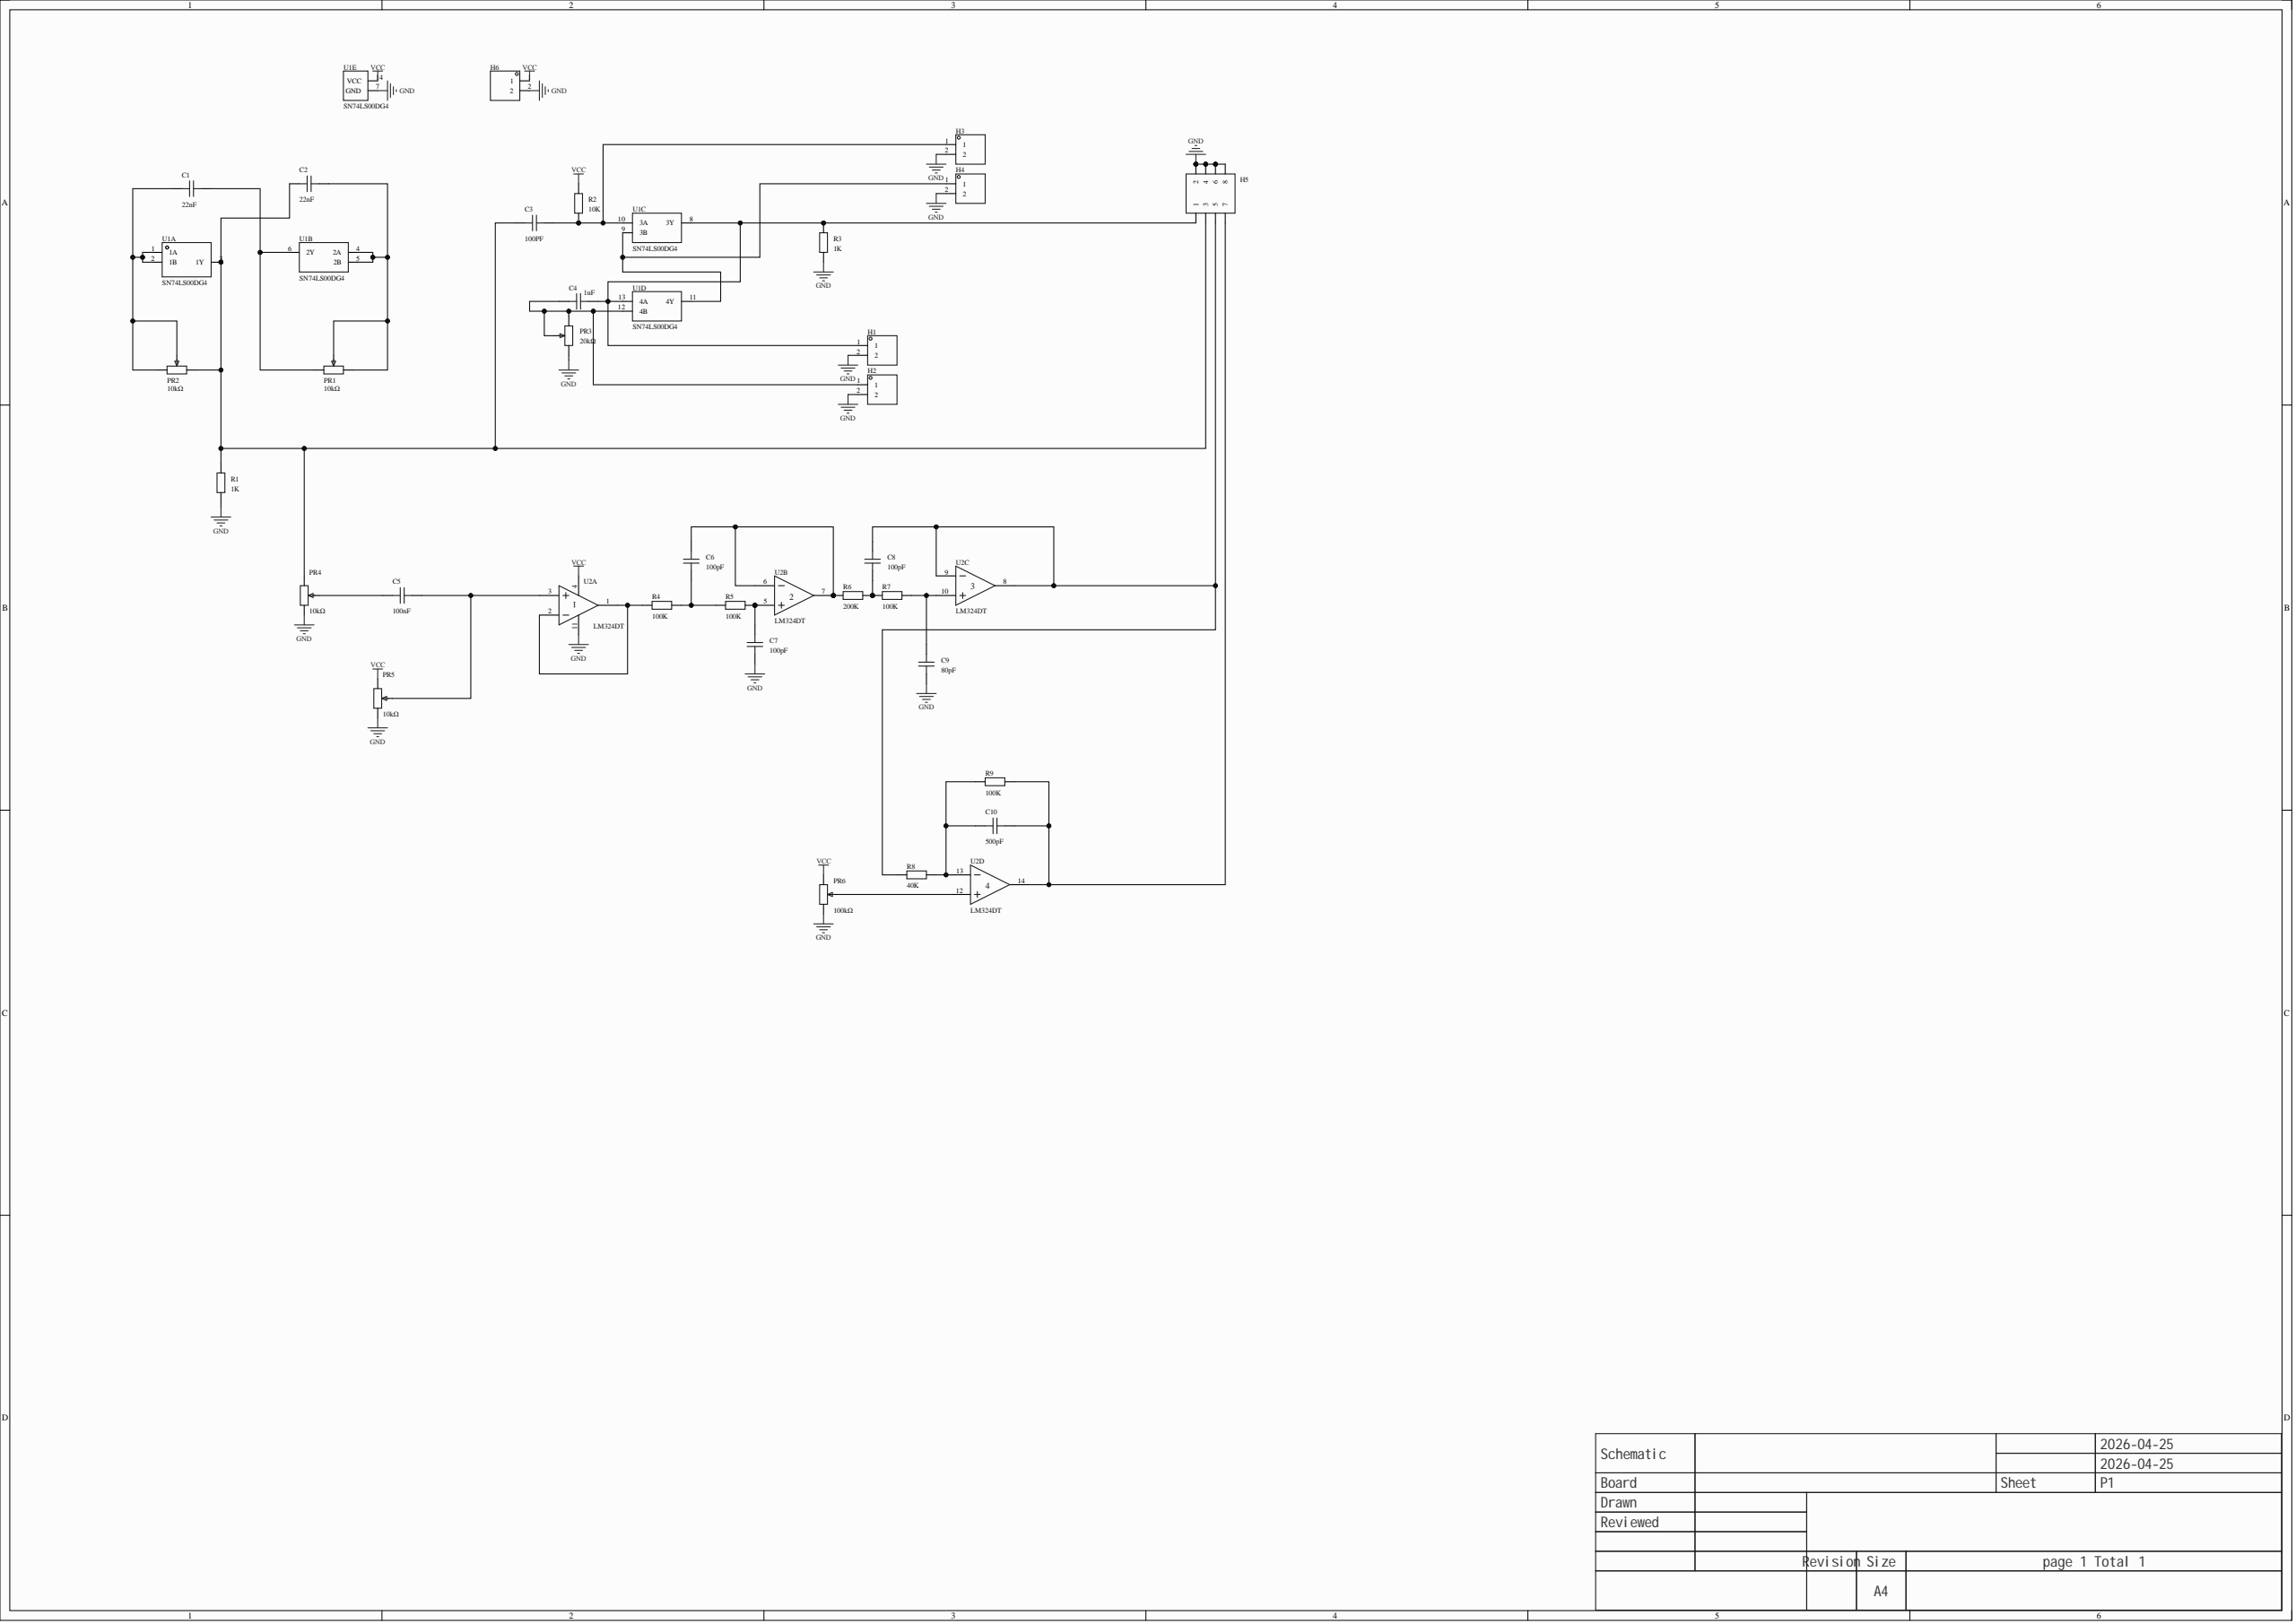Circuit board | Altium Designer | 33 parts | 22 nets
Bill of materials:
Comment,Description,Designator,Footprint,LibRef,Quantity
"22nF","","C1, C2","C0603","CAP_0603","2"
"100PF","","C3, C6, C7, C8","C0603","CAP_0603","4"
"1nF","","C4","C0603","CAP_0603","1"
"100nF","","C5","C0603","CAP_0603","1"
"80pF","","C9","C0603","CAP_0603","1"
"500pF","","C10","C0603","CAP_0603","1"
"","","H1, H2, H3, H4, H6","HDR-TH_2P-P2.54-V-M-1","HDR-M_2.54_1x2P","5"
"","","H5","HDR-TH_8P-P2.54-V-F-R2-C4-S2.54-1","HDR-F_2.54_2x4","1"
"10kΩ","","PR1, PR2, PR4, PR5","R_3296","R_3296","4"
"20kΩ","","PR3","R_3296","R_3296","1"
"100kΩ","","PR6","R_3296","R_3296","1"
"1K","","R1, R3","R0603","Res_0603","2"
"10K","","R2","R0603","Res_0603","1"
"100K","","R4, R5, R7, R9","R0603","Res_0603","4"
"200K","","R6","R0603","Res_0603","1"
"40K","","R8","R0603","Res_0603","1"
"SN74LS00DG4","","U1","SOIC-14_L8.7-W3.9-P1.27-LS6.0-BL","SN74LS00DG4","1"
"LM324DT","放大器数:4;轨到轨:-;增益带宽积(GBW):1.3MHz;输入失调电压(Vos):5mV;压摆率(SR):400V/ms;输入偏置电流(Ib):300nA;","U2","SOIC-14_L8.7-W3.9-P1.27-LS6.0-BL","LM324DT","1"
Netlist (Protel format):
[
C1
C0603
22nF



]
[
C2
C0603
22nF



]
[
C3
C0603
100PF



]
[
C4
C0603
1nF



]
[
C5
C0603
100nF



]
[
C6
C0603
100pF



]
[
C7
C0603
100pF



]
[
C8
C0603
100pF



]
[
C9
C0603
80pF



]
[
C10
C0603
500pF



]
[
H1
HDR-TH_2P-P2.54-V-M-1




]
[
H2
HDR-TH_2P-P2.54-V-M-1




]
[
H3
HDR-TH_2P-P2.54-V-M-1




]
[
H4
HDR-TH_2P-P2.54-V-M-1




]
[
H5
HDR-TH_8P-P2.54-V-F-R2-C4-S2.54-1




]
[
H6
HDR-TH_2P-P2.54-V-M-1




]
[
PR1
R_3296
10kΩ



]
[
PR2
R_3296
10kΩ



]
[
PR3
R_3296
20kΩ



]
[
PR4
R_3296
10kΩ



]
[
PR5
R_3296
10kΩ



]
[
PR6
R_3296
100kΩ



]
[
R1
R0603
1K



]
[
R2
R0603
10K



]
[
R3
R0603
1K



]
[
R4
R0603
100K



]
[
R5
R0603
100K



]
[
R6
R0603
200K



]
[
R7
R0603
100K



]
[
R8
R0603
40K



]
[
R9
R0603
100K



]
[
U1
SOIC-14_L8.7-W3.9-P1.27-LS6.0-BL
SN74LS00DG4



]
[
U2
SOIC-14_L8.7-W3.9-P1.27-LS6.0-BL
LM324DT



]
(
VCC
H6-1
PR5-3
PR6-3
R2-2
U1-14
U2-4
)
(
NetR4_1
R4-1
U2-1
U2-2
)
(
NetPR6_2
PR6-2
U2-12
)
(
NetH4_1
H4-1
U1-9
U1-11
)
(
NetC10_2
C10-2
R8-2
R9-1
U2-13
)
(
NetC10_1
C10-1
H5-7
R9-2
U2-14
)
(
NetC9_2
C9-2
R7-2
U2-10
)
(
NetC8_2
C8-2
H5-5
R8-1
U2-8
U2-9
)
(
NetC8_1
C8-1
R6-2
R7-1
)
(
NetC7_2
C7-2
R5-2
U2-5
)
(
NetC6_2
C6-2
R6-1
U2-6
U2-7
)
(
NetC6_1
C6-1
R4-2
R5-1
)
(
NetC5_2
C5-2
PR5-2
U2-3
)
(
NetC5_1
C5-1
PR4-2
)
(
NetC4_2
C4-2
H1-1
H5-1
R3-2
U1-8
U1-13
)
(
NetC4_1
C4-1
H2-1
PR3-1
PR3-2
U1-12
)
(
NetC3_2
C3-2
H3-1
R2-1
U1-10
)
(
NetC2_2
C2-2
PR1-1
PR1-2
U1-4
U1-5
)
(
NetC2_1
C2-1
C3-1
H5-3
PR2-1
PR4-3
R1-2
U1-3
)
(
NetC1_2
C1-2
PR1-3
U1-6
)
(
NetC1_1
C1-1
PR2-2
PR2-3
U1-1
U1-2
)
(
GND
C7-1
C9-1
H1-2
H2-2
H3-2
H4-2
H5-2
H5-4
H5-6
H5-8
H6-2
PR3-3
PR4-1
PR5-1
PR6-1
R1-1
R3-1
U1-7
U2-11
)